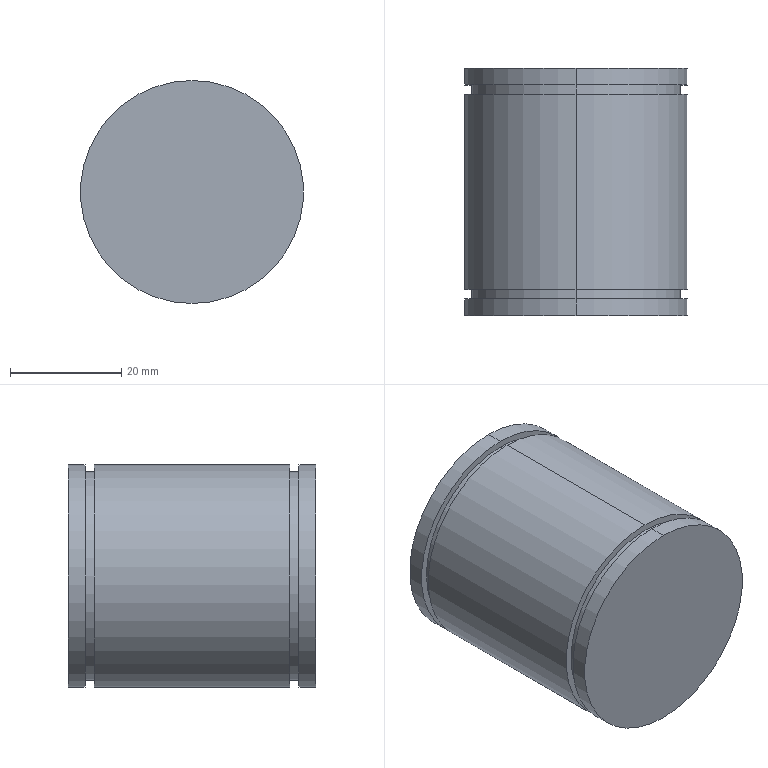Part | SolidWorks | features Extrusion 1, MirrorPattern 1, RevCut 1 | 1 solid | 16 faces | box 40 x 44.4 x 40 mm | volume 55277 mm3 | cylinder 10 | plane 6 | commonest cylinder face diameters 40 x6 37.5 x4
STEP:
#1=CARTESIAN_POINT('',(0.,44.4,20.));
#2=VERTEX_POINT('',#1);
#3=CARTESIAN_POINT('',(0.,44.4,-20.));
#4=VERTEX_POINT('',#3);
#5=CARTESIAN_POINT('',(0.,44.4,0.));
#6=DIRECTION('',(0.,1.,0.));
#7=DIRECTION('',(0.,0.,1.));
#8=AXIS2_PLACEMENT_3D('',#5,#6,#7);
#9=CIRCLE('',#8,20.);
#10=EDGE_CURVE('',#2,#4,#9,.T.);
#11=ORIENTED_EDGE('',*,*,#10,.F.);
#12=CARTESIAN_POINT('',(0.,41.4,20.));
#13=VERTEX_POINT('',#12);
#14=CARTESIAN_POINT('',(0.,44.4,20.));
#15=DIRECTION('',(0.,-1.,0.));
#16=VECTOR('',#15,1000.);
#17=LINE('',#14,#16);
#18=EDGE_CURVE('',#2,#13,#17,.T.);
#19=ORIENTED_EDGE('',*,*,#18,.T.);
#20=CARTESIAN_POINT('',(0.,41.4,-20.));
#21=VERTEX_POINT('',#20);
#22=CARTESIAN_POINT('',(0.,41.4,0.));
#23=DIRECTION('',(0.,1.,0.));
#24=DIRECTION('',(0.,0.,1.));
#25=AXIS2_PLACEMENT_3D('',#22,#23,#24);
#26=CIRCLE('',#25,20.);
#27=EDGE_CURVE('',#13,#21,#26,.T.);
#28=ORIENTED_EDGE('',*,*,#27,.T.);
#29=CARTESIAN_POINT('',(0.,44.4,-20.));
#30=DIRECTION('',(0.,-1.,0.));
#31=VECTOR('',#30,1000.);
#32=LINE('',#29,#31);
#33=EDGE_CURVE('',#4,#21,#32,.T.);
#34=ORIENTED_EDGE('',*,*,#33,.F.);
#35=EDGE_LOOP('',(#11,#19,#28,#34));
#36=FACE_OUTER_BOUND('',#35,.T.);
#37=CARTESIAN_POINT('',(0.,44.4,0.));
#38=DIRECTION('',(0.,-1.,0.));
#39=DIRECTION('',(0.,0.,-1.));
#40=AXIS2_PLACEMENT_3D('',#37,#38,#39);
#41=CYLINDRICAL_SURFACE('',#40,20.);
#42=ADVANCED_FACE('',(#36),#41,.T.);
#43=CARTESIAN_POINT('',(0.,41.4,-18.75));
#44=VERTEX_POINT('',#43);
#45=CARTESIAN_POINT('',(0.,41.4,18.75));
#46=VERTEX_POINT('',#45);
#47=CARTESIAN_POINT('',(0.,41.4,0.));
#48=DIRECTION('',(0.,1.,0.));
#49=DIRECTION('',(0.,0.,1.));
#50=AXIS2_PLACEMENT_3D('',#47,#48,#49);
#51=CIRCLE('',#50,18.75);
#52=EDGE_CURVE('',#44,#46,#51,.T.);
#53=ORIENTED_EDGE('',*,*,#52,.F.);
#54=CARTESIAN_POINT('',(0.,39.7,-18.75));
#55=VERTEX_POINT('',#54);
#56=CARTESIAN_POINT('',(0.,0.,-18.75));
#57=DIRECTION('',(0.,-1.,0.));
#58=VECTOR('',#57,1000.);
#59=LINE('',#56,#58);
#60=EDGE_CURVE('',#44,#55,#59,.T.);
#61=ORIENTED_EDGE('',*,*,#60,.T.);
#62=CARTESIAN_POINT('',(0.,39.7,18.75));
#63=VERTEX_POINT('',#62);
#64=CARTESIAN_POINT('',(0.,39.7,0.));
#65=DIRECTION('',(0.,1.,0.));
#66=DIRECTION('',(0.,0.,1.));
#67=AXIS2_PLACEMENT_3D('',#64,#65,#66);
#68=CIRCLE('',#67,18.75);
#69=EDGE_CURVE('',#55,#63,#68,.T.);
#70=ORIENTED_EDGE('',*,*,#69,.T.);
#71=CARTESIAN_POINT('',(0.,0.,18.75));
#72=DIRECTION('',(0.,-1.,0.));
#73=VECTOR('',#72,1000.);
#74=LINE('',#71,#73);
#75=EDGE_CURVE('',#46,#63,#74,.T.);
#76=ORIENTED_EDGE('',*,*,#75,.F.);
#77=EDGE_LOOP('',(#53,#61,#70,#76));
#78=FACE_OUTER_BOUND('',#77,.T.);
#79=CARTESIAN_POINT('',(0.,0.,0.));
#80=DIRECTION('',(0.,-1.,0.));
#81=DIRECTION('',(0.,0.,1.));
#82=AXIS2_PLACEMENT_3D('',#79,#80,#81);
#83=CYLINDRICAL_SURFACE('',#82,18.75);
#84=ADVANCED_FACE('',(#78),#83,.T.);
#85=CARTESIAN_POINT('',(0.,3.,-20.));
#86=VERTEX_POINT('',#85);
#87=CARTESIAN_POINT('',(0.,3.,20.));
#88=VERTEX_POINT('',#87);
#89=CARTESIAN_POINT('',(0.,3.,0.));
#90=DIRECTION('',(0.,-1.,0.));
#91=DIRECTION('',(0.,0.,-1.));
#92=AXIS2_PLACEMENT_3D('',#89,#90,#91);
#93=CIRCLE('',#92,20.);
#94=EDGE_CURVE('',#86,#88,#93,.T.);
#95=ORIENTED_EDGE('',*,*,#94,.T.);
#96=CARTESIAN_POINT('',(0.,0.,20.));
#97=VERTEX_POINT('',#96);
#98=CARTESIAN_POINT('',(0.,44.4,20.));
#99=DIRECTION('',(0.,-1.,0.));
#100=VECTOR('',#99,1000.);
#101=LINE('',#98,#100);
#102=EDGE_CURVE('',#88,#97,#101,.T.);
#103=ORIENTED_EDGE('',*,*,#102,.T.);
#104=CARTESIAN_POINT('',(0.,0.,-20.));
#105=VERTEX_POINT('',#104);
#106=CARTESIAN_POINT('',(0.,0.,0.));
#107=DIRECTION('',(0.,1.,0.));
#108=DIRECTION('',(0.,0.,1.));
#109=AXIS2_PLACEMENT_3D('',#106,#107,#108);
#110=CIRCLE('',#109,20.);
#111=EDGE_CURVE('',#97,#105,#110,.T.);
#112=ORIENTED_EDGE('',*,*,#111,.T.);
#113=CARTESIAN_POINT('',(0.,44.4,-20.));
#114=DIRECTION('',(0.,-1.,0.));
#115=VECTOR('',#114,1000.);
#116=LINE('',#113,#115);
#117=EDGE_CURVE('',#86,#105,#116,.T.);
#118=ORIENTED_EDGE('',*,*,#117,.F.);
#119=EDGE_LOOP('',(#95,#103,#112,#118));
#120=FACE_OUTER_BOUND('',#119,.T.);
#121=CARTESIAN_POINT('',(0.,44.4,0.));
#122=DIRECTION('',(0.,-1.,0.));
#123=DIRECTION('',(0.,0.,-1.));
#124=AXIS2_PLACEMENT_3D('',#121,#122,#123);
#125=CYLINDRICAL_SURFACE('',#124,20.);
#126=ADVANCED_FACE('',(#120),#125,.T.);
#127=CARTESIAN_POINT('',(0.,3.,18.75));
#128=VERTEX_POINT('',#127);
#129=CARTESIAN_POINT('',(0.,3.,-18.75));
#130=VERTEX_POINT('',#129);
#131=CARTESIAN_POINT('',(0.,3.,0.));
#132=DIRECTION('',(0.,1.,0.));
#133=DIRECTION('',(0.,0.,1.));
#134=AXIS2_PLACEMENT_3D('',#131,#132,#133);
#135=CIRCLE('',#134,18.75);
#136=EDGE_CURVE('',#128,#130,#135,.T.);
#137=ORIENTED_EDGE('',*,*,#136,.T.);
#138=CARTESIAN_POINT('',(0.,4.7,-18.75));
#139=VERTEX_POINT('',#138);
#140=CARTESIAN_POINT('',(0.,44.4,-18.75));
#141=DIRECTION('',(0.,1.,0.));
#142=VECTOR('',#141,1000.);
#143=LINE('',#140,#142);
#144=EDGE_CURVE('',#130,#139,#143,.T.);
#145=ORIENTED_EDGE('',*,*,#144,.T.);
#146=CARTESIAN_POINT('',(0.,4.7,18.75));
#147=VERTEX_POINT('',#146);
#148=CARTESIAN_POINT('',(0.,4.7,0.));
#149=DIRECTION('',(0.,1.,0.));
#150=DIRECTION('',(0.,0.,1.));
#151=AXIS2_PLACEMENT_3D('',#148,#149,#150);
#152=CIRCLE('',#151,18.75);
#153=EDGE_CURVE('',#147,#139,#152,.T.);
#154=ORIENTED_EDGE('',*,*,#153,.F.);
#155=CARTESIAN_POINT('',(0.,44.4,18.75));
#156=DIRECTION('',(0.,1.,0.));
#157=VECTOR('',#156,1000.);
#158=LINE('',#155,#157);
#159=EDGE_CURVE('',#128,#147,#158,.T.);
#160=ORIENTED_EDGE('',*,*,#159,.F.);
#161=EDGE_LOOP('',(#137,#145,#154,#160));
#162=FACE_OUTER_BOUND('',#161,.T.);
#163=CARTESIAN_POINT('',(0.,44.4,0.));
#164=DIRECTION('',(0.,1.,0.));
#165=DIRECTION('',(0.,0.,1.));
#166=AXIS2_PLACEMENT_3D('',#163,#164,#165);
#167=CYLINDRICAL_SURFACE('',#166,18.75);
#168=ADVANCED_FACE('',(#162),#167,.T.);
#169=CARTESIAN_POINT('',(0.,39.7,-20.));
#170=VERTEX_POINT('',#169);
#171=CARTESIAN_POINT('',(0.,39.7,20.));
#172=VERTEX_POINT('',#171);
#173=CARTESIAN_POINT('',(0.,39.7,0.));
#174=DIRECTION('',(0.,-1.,0.));
#175=DIRECTION('',(0.,0.,-1.));
#176=AXIS2_PLACEMENT_3D('',#173,#174,#175);
#177=CIRCLE('',#176,20.);
#178=EDGE_CURVE('',#170,#172,#177,.T.);
#179=ORIENTED_EDGE('',*,*,#178,.T.);
#180=CARTESIAN_POINT('',(0.,4.7,20.));
#181=VERTEX_POINT('',#180);
#182=CARTESIAN_POINT('',(0.,44.4,20.));
#183=DIRECTION('',(0.,-1.,0.));
#184=VECTOR('',#183,1000.);
#185=LINE('',#182,#184);
#186=EDGE_CURVE('',#172,#181,#185,.T.);
#187=ORIENTED_EDGE('',*,*,#186,.T.);
#188=CARTESIAN_POINT('',(0.,4.7,-20.));
#189=VERTEX_POINT('',#188);
#190=CARTESIAN_POINT('',(0.,4.7,0.));
#191=DIRECTION('',(0.,1.,0.));
#192=DIRECTION('',(0.,0.,1.));
#193=AXIS2_PLACEMENT_3D('',#190,#191,#192);
#194=CIRCLE('',#193,20.);
#195=EDGE_CURVE('',#181,#189,#194,.T.);
#196=ORIENTED_EDGE('',*,*,#195,.T.);
#197=CARTESIAN_POINT('',(0.,44.4,-20.));
#198=DIRECTION('',(0.,-1.,0.));
#199=VECTOR('',#198,1000.);
#200=LINE('',#197,#199);
#201=EDGE_CURVE('',#170,#189,#200,.T.);
#202=ORIENTED_EDGE('',*,*,#201,.F.);
#203=EDGE_LOOP('',(#179,#187,#196,#202));
#204=FACE_OUTER_BOUND('',#203,.T.);
#205=CARTESIAN_POINT('',(0.,44.4,0.));
#206=DIRECTION('',(0.,-1.,0.));
#207=DIRECTION('',(0.,0.,-1.));
#208=AXIS2_PLACEMENT_3D('',#205,#206,#207);
#209=CYLINDRICAL_SURFACE('',#208,20.);
#210=ADVANCED_FACE('',(#204),#209,.T.);
#211=ORIENTED_EDGE('',*,*,#186,.F.);
#212=CARTESIAN_POINT('',(0.,39.7,0.));
#213=DIRECTION('',(0.,-1.,0.));
#214=DIRECTION('',(0.,0.,-1.));
#215=AXIS2_PLACEMENT_3D('',#212,#213,#214);
#216=CIRCLE('',#215,20.);
#217=EDGE_CURVE('',#172,#170,#216,.T.);
#218=ORIENTED_EDGE('',*,*,#217,.T.);
#219=ORIENTED_EDGE('',*,*,#201,.T.);
#220=CARTESIAN_POINT('',(0.,4.7,0.));
#221=DIRECTION('',(0.,1.,0.));
#222=DIRECTION('',(0.,0.,1.));
#223=AXIS2_PLACEMENT_3D('',#220,#221,#222);
#224=CIRCLE('',#223,20.);
#225=EDGE_CURVE('',#189,#181,#224,.T.);
#226=ORIENTED_EDGE('',*,*,#225,.T.);
#227=EDGE_LOOP('',(#211,#218,#219,#226));
#228=FACE_OUTER_BOUND('',#227,.T.);
#229=CARTESIAN_POINT('',(0.,44.4,0.));
#230=DIRECTION('',(0.,-1.,0.));
#231=DIRECTION('',(0.,0.,-1.));
#232=AXIS2_PLACEMENT_3D('',#229,#230,#231);
#233=CYLINDRICAL_SURFACE('',#232,20.);
#234=ADVANCED_FACE('',(#228),#233,.T.);
#235=ORIENTED_EDGE('',*,*,#153,.T.);
#236=CARTESIAN_POINT('',(0.,4.7,0.));
#237=DIRECTION('',(0.,1.,0.));
#238=DIRECTION('',(0.,0.,1.));
#239=AXIS2_PLACEMENT_3D('',#236,#237,#238);
#240=CIRCLE('',#239,18.75);
#241=EDGE_CURVE('',#139,#147,#240,.T.);
#242=ORIENTED_EDGE('',*,*,#241,.T.);
#243=EDGE_LOOP('',(#235,#242));
#244=FACE_BOUND('',#243,.T.);
#245=ORIENTED_EDGE('',*,*,#225,.F.);
#246=ORIENTED_EDGE('',*,*,#195,.F.);
#247=EDGE_LOOP('',(#245,#246));
#248=FACE_OUTER_BOUND('',#247,.T.);
#249=CARTESIAN_POINT('',(-21.29,4.7,0.));
#250=DIRECTION('',(0.,1.,0.));
#251=DIRECTION('',(0.,0.,1.));
#252=AXIS2_PLACEMENT_3D('',#249,#250,#251);
#253=PLANE('',#252);
#254=ADVANCED_FACE('',(#244,#248),#253,.F.);
#255=ORIENTED_EDGE('',*,*,#136,.F.);
#256=CARTESIAN_POINT('',(0.,3.,0.));
#257=DIRECTION('',(0.,1.,0.));
#258=DIRECTION('',(0.,0.,1.));
#259=AXIS2_PLACEMENT_3D('',#256,#257,#258);
#260=CIRCLE('',#259,18.75);
#261=EDGE_CURVE('',#130,#128,#260,.T.);
#262=ORIENTED_EDGE('',*,*,#261,.F.);
#263=EDGE_LOOP('',(#255,#262));
#264=FACE_BOUND('',#263,.T.);
#265=ORIENTED_EDGE('',*,*,#94,.F.);
#266=CARTESIAN_POINT('',(0.,3.,0.));
#267=DIRECTION('',(0.,-1.,0.));
#268=DIRECTION('',(0.,0.,-1.));
#269=AXIS2_PLACEMENT_3D('',#266,#267,#268);
#270=CIRCLE('',#269,20.);
#271=EDGE_CURVE('',#88,#86,#270,.T.);
#272=ORIENTED_EDGE('',*,*,#271,.F.);
#273=EDGE_LOOP('',(#265,#272));
#274=FACE_OUTER_BOUND('',#273,.T.);
#275=CARTESIAN_POINT('',(-21.29,3.,0.));
#276=DIRECTION('',(0.,-1.,0.));
#277=DIRECTION('',(0.,0.,-1.));
#278=AXIS2_PLACEMENT_3D('',#275,#276,#277);
#279=PLANE('',#278);
#280=ADVANCED_FACE('',(#264,#274),#279,.F.);
#281=ORIENTED_EDGE('',*,*,#144,.F.);
#282=ORIENTED_EDGE('',*,*,#261,.T.);
#283=ORIENTED_EDGE('',*,*,#159,.T.);
#284=ORIENTED_EDGE('',*,*,#241,.F.);
#285=EDGE_LOOP('',(#281,#282,#283,#284));
#286=FACE_OUTER_BOUND('',#285,.T.);
#287=CARTESIAN_POINT('',(0.,44.4,0.));
#288=DIRECTION('',(0.,1.,0.));
#289=DIRECTION('',(0.,0.,1.));
#290=AXIS2_PLACEMENT_3D('',#287,#288,#289);
#291=CYLINDRICAL_SURFACE('',#290,18.75);
#292=ADVANCED_FACE('',(#286),#291,.T.);
#293=CARTESIAN_POINT('',(0.,0.,0.));
#294=DIRECTION('',(0.,1.,0.));
#295=DIRECTION('',(0.,0.,1.));
#296=AXIS2_PLACEMENT_3D('',#293,#294,#295);
#297=CIRCLE('',#296,20.);
#298=EDGE_CURVE('',#105,#97,#297,.T.);
#299=ORIENTED_EDGE('',*,*,#298,.F.);
#300=ORIENTED_EDGE('',*,*,#111,.F.);
#301=EDGE_LOOP('',(#299,#300));
#302=FACE_OUTER_BOUND('',#301,.T.);
#303=CARTESIAN_POINT('',(0.,0.,0.));
#304=DIRECTION('',(0.,1.,0.));
#305=DIRECTION('',(0.,0.,1.));
#306=AXIS2_PLACEMENT_3D('',#303,#304,#305);
#307=PLANE('',#306);
#308=ADVANCED_FACE('',(#302),#307,.F.);
#309=ORIENTED_EDGE('',*,*,#102,.F.);
#310=ORIENTED_EDGE('',*,*,#271,.T.);
#311=ORIENTED_EDGE('',*,*,#117,.T.);
#312=ORIENTED_EDGE('',*,*,#298,.T.);
#313=EDGE_LOOP('',(#309,#310,#311,#312));
#314=FACE_OUTER_BOUND('',#313,.T.);
#315=CARTESIAN_POINT('',(0.,44.4,0.));
#316=DIRECTION('',(0.,-1.,0.));
#317=DIRECTION('',(0.,0.,-1.));
#318=AXIS2_PLACEMENT_3D('',#315,#316,#317);
#319=CYLINDRICAL_SURFACE('',#318,20.);
#320=ADVANCED_FACE('',(#314),#319,.T.);
#321=CARTESIAN_POINT('',(0.,39.7,0.));
#322=DIRECTION('',(0.,1.,0.));
#323=DIRECTION('',(0.,0.,1.));
#324=AXIS2_PLACEMENT_3D('',#321,#322,#323);
#325=CIRCLE('',#324,18.75);
#326=EDGE_CURVE('',#63,#55,#325,.T.);
#327=ORIENTED_EDGE('',*,*,#326,.F.);
#328=ORIENTED_EDGE('',*,*,#69,.F.);
#329=EDGE_LOOP('',(#327,#328));
#330=FACE_BOUND('',#329,.T.);
#331=ORIENTED_EDGE('',*,*,#178,.F.);
#332=ORIENTED_EDGE('',*,*,#217,.F.);
#333=EDGE_LOOP('',(#331,#332));
#334=FACE_OUTER_BOUND('',#333,.T.);
#335=CARTESIAN_POINT('',(-21.29,39.7,0.));
#336=DIRECTION('',(0.,-1.,0.));
#337=DIRECTION('',(0.,0.,1.));
#338=AXIS2_PLACEMENT_3D('',#335,#336,#337);
#339=PLANE('',#338);
#340=ADVANCED_FACE('',(#330,#334),#339,.F.);
#341=CARTESIAN_POINT('',(0.,41.4,0.));
#342=DIRECTION('',(0.,1.,0.));
#343=DIRECTION('',(0.,0.,1.));
#344=AXIS2_PLACEMENT_3D('',#341,#342,#343);
#345=CIRCLE('',#344,18.75);
#346=EDGE_CURVE('',#46,#44,#345,.T.);
#347=ORIENTED_EDGE('',*,*,#346,.T.);
#348=ORIENTED_EDGE('',*,*,#52,.T.);
#349=EDGE_LOOP('',(#347,#348));
#350=FACE_BOUND('',#349,.T.);
#351=CARTESIAN_POINT('',(0.,41.4,0.));
#352=DIRECTION('',(0.,1.,0.));
#353=DIRECTION('',(0.,0.,1.));
#354=AXIS2_PLACEMENT_3D('',#351,#352,#353);
#355=CIRCLE('',#354,20.);
#356=EDGE_CURVE('',#21,#13,#355,.T.);
#357=ORIENTED_EDGE('',*,*,#356,.F.);
#358=ORIENTED_EDGE('',*,*,#27,.F.);
#359=EDGE_LOOP('',(#357,#358));
#360=FACE_OUTER_BOUND('',#359,.T.);
#361=CARTESIAN_POINT('',(-21.29,41.4,0.));
#362=DIRECTION('',(0.,1.,0.));
#363=DIRECTION('',(0.,0.,-1.));
#364=AXIS2_PLACEMENT_3D('',#361,#362,#363);
#365=PLANE('',#364);
#366=ADVANCED_FACE('',(#350,#360),#365,.F.);
#367=ORIENTED_EDGE('',*,*,#60,.F.);
#368=ORIENTED_EDGE('',*,*,#346,.F.);
#369=ORIENTED_EDGE('',*,*,#75,.T.);
#370=ORIENTED_EDGE('',*,*,#326,.T.);
#371=EDGE_LOOP('',(#367,#368,#369,#370));
#372=FACE_OUTER_BOUND('',#371,.T.);
#373=CARTESIAN_POINT('',(0.,0.,0.));
#374=DIRECTION('',(0.,-1.,0.));
#375=DIRECTION('',(0.,0.,1.));
#376=AXIS2_PLACEMENT_3D('',#373,#374,#375);
#377=CYLINDRICAL_SURFACE('',#376,18.75);
#378=ADVANCED_FACE('',(#372),#377,.T.);
#379=CARTESIAN_POINT('',(0.,44.4,0.));
#380=DIRECTION('',(0.,1.,0.));
#381=DIRECTION('',(0.,0.,1.));
#382=AXIS2_PLACEMENT_3D('',#379,#380,#381);
#383=CIRCLE('',#382,20.);
#384=EDGE_CURVE('',#4,#2,#383,.T.);
#385=ORIENTED_EDGE('',*,*,#384,.T.);
#386=ORIENTED_EDGE('',*,*,#10,.T.);
#387=EDGE_LOOP('',(#385,#386));
#388=FACE_OUTER_BOUND('',#387,.T.);
#389=CARTESIAN_POINT('',(0.,44.4,0.));
#390=DIRECTION('',(0.,1.,0.));
#391=DIRECTION('',(0.,0.,1.));
#392=AXIS2_PLACEMENT_3D('',#389,#390,#391);
#393=PLANE('',#392);
#394=ADVANCED_FACE('',(#388),#393,.T.);
#395=ORIENTED_EDGE('',*,*,#18,.F.);
#396=ORIENTED_EDGE('',*,*,#384,.F.);
#397=ORIENTED_EDGE('',*,*,#33,.T.);
#398=ORIENTED_EDGE('',*,*,#356,.T.);
#399=EDGE_LOOP('',(#395,#396,#397,#398));
#400=FACE_OUTER_BOUND('',#399,.T.);
#401=CARTESIAN_POINT('',(0.,44.4,0.));
#402=DIRECTION('',(0.,-1.,0.));
#403=DIRECTION('',(0.,0.,-1.));
#404=AXIS2_PLACEMENT_3D('',#401,#402,#403);
#405=CYLINDRICAL_SURFACE('',#404,20.);
#406=ADVANCED_FACE('',(#400),#405,.T.);
#407=CLOSED_SHELL('',(#42,#84,#126,#168,#210,#234,#254,#280,#292,#308,#320,#340,#366,#378,#394,#406));
#408=MANIFOLD_SOLID_BREP('',#407);
#409=CARTESIAN_POINT('',(0.,0.,0.));
#410=DIRECTION('',(0.,0.,1.));
#411=DIRECTION('',(1.,0.,0.));
#412=AXIS2_PLACEMENT_3D('',#409,#410,#411);
#413=(LENGTH_UNIT()NAMED_UNIT(*)SI_UNIT(.MILLI.,.METRE.));
#414=UNCERTAINTY_MEASURE_WITH_UNIT(LENGTH_MEASURE(0.00001),#413,'','');
#415=(NAMED_UNIT(*)PLANE_ANGLE_UNIT()SI_UNIT($,.RADIAN.));
#416=(NAMED_UNIT(*)SI_UNIT($,.STERADIAN.)SOLID_ANGLE_UNIT());
#417=(GEOMETRIC_REPRESENTATION_CONTEXT(3)GLOBAL_UNCERTAINTY_ASSIGNED_CONTEXT((#414))GLOBAL_UNIT_ASSIGNED_CONTEXT((#413,#415,#416))REPRESENTATION_CONTEXT('',''));
#418=ADVANCED_BREP_SHAPE_REPRESENTATION('',(#408,#412),#417);